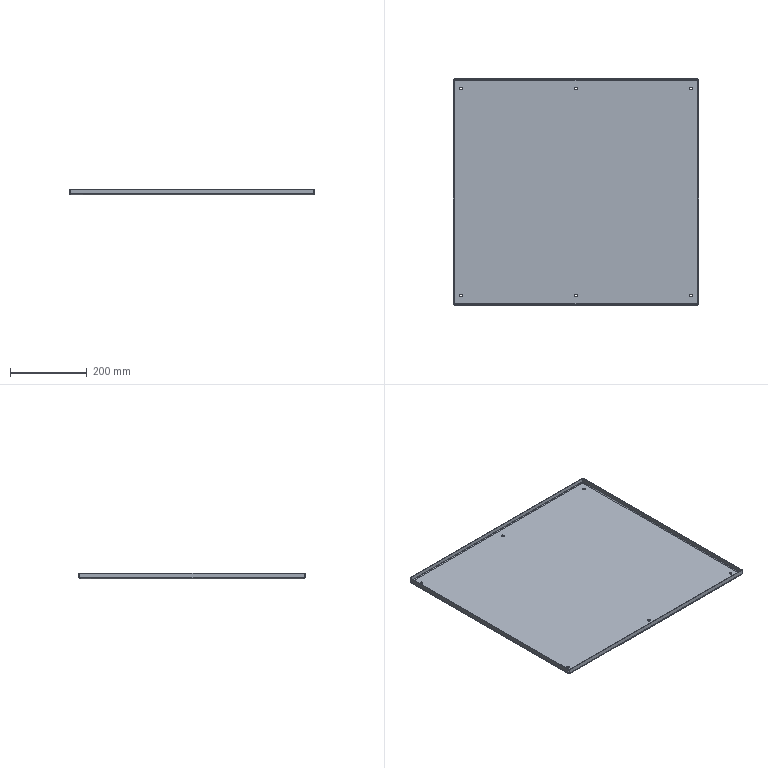Part | SolidWorks | features EdgeFlange 1, FlatPattern 1, HoleWzd 1, SMBaseFlange 1, SheetMetal 1 | 1 solid | 50 faces | box 640 x 590 x 15 mm | volume 811762 mm3 | plane 22 | cylinder 20 | spline 8 | commonest cylinder face diameters 7 x12 4 x4 8 x4